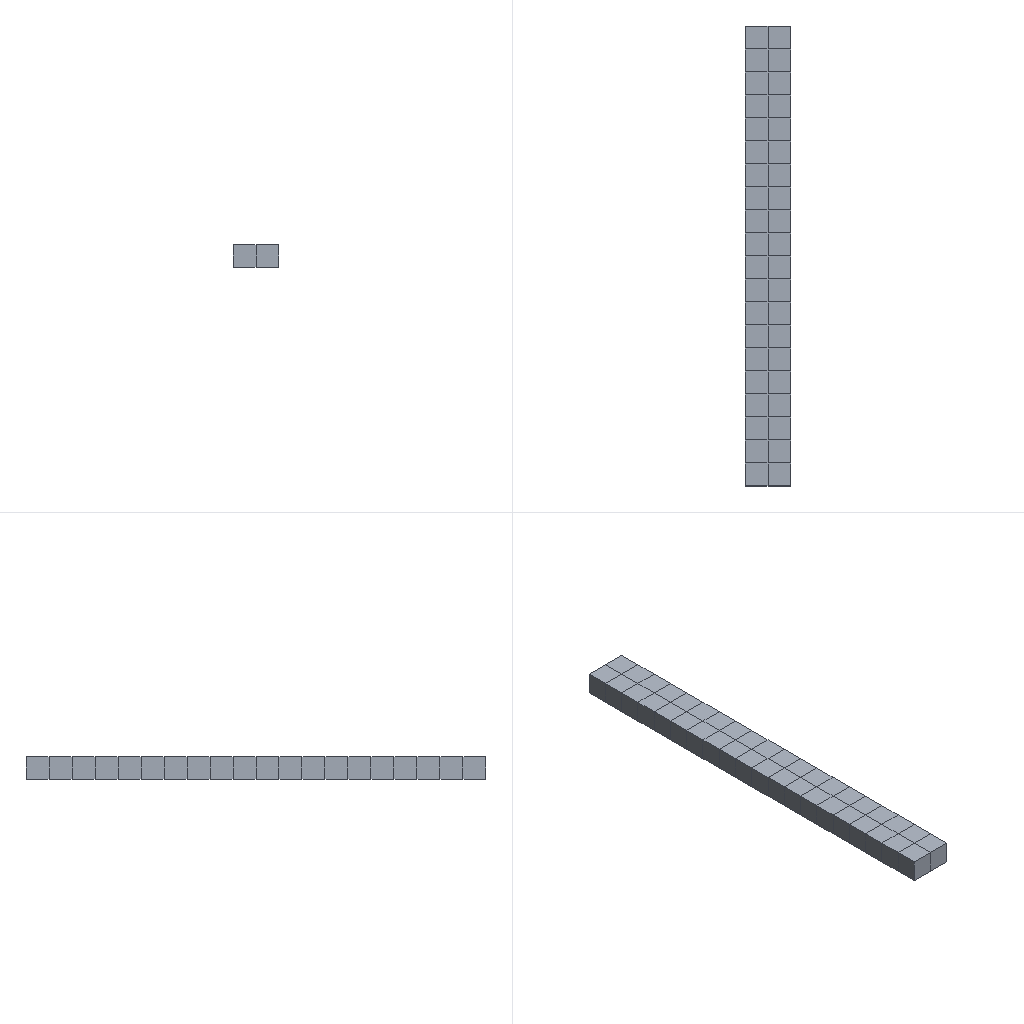Simulation study | ansys workbench
Ansys APDL input file, long lists of numbers shortened:
/batch
/config,noeldb,1     ! force off writing results to database
*get,_wallstrt,active,,time,wall
! ANSYS input file written by Workbench version 2022 R1
! File used for geometry attach: C:\Users\Administrator\AppData\Local\Temp\WB_Administrator_19516_2\wbnew_files\dp0\SYS\DM\SYS.scdoc
/title,wbnew--____ (A5)
! ****** Begin Custom Load Command Snippet ******
/COM, ACT Extensions:
/COM,     LSDYNA, 2021.1
/COM,
! ****** End   Custom Load Command Snippet ******
*DIM,_wb_ProjectScratch_dir,string,248
_wb_ProjectScratch_dir(1) = 'C:\Users\Administrator\AppData\Local\Temp\WB_Administrator_19516_2\_ProjectScratch\Scr58CE\'
*DIM,_wb_SolverFiles_dir,string,248
_wb_SolverFiles_dir(1) = 'C:\Users\Administrator\AppData\Local\Temp\WB_Administrator_19516_2\wbnew_files\dp0\SYS\MECH\'
*DIM,_wb_userfiles_dir,string,248
_wb_userfiles_dir(1) = 'C:\Users\Administrator\AppData\Local\Temp\WB_Administrator_19516_2\wbnew_files\user_files\'
/com,--- Data in consistent NMM units. See Solving Units in the help system for more information.
/units,MPA
/nopr
/wb,file,start              !  signify a WB generated input file
/prep7
! Turn off shape checking because checks already performed inside WB mesher.
! See help system for more information.
SHPP,OFF,,NOWARN
/nolist
etcon,set             ! allow ANSYS to choose best KEYOP's for 180x elements, resets any applicable keyopt to MAPDL defaults
/com,*********** Nodes for the whole assembly ***********
nblock,3,,1377
(1i9,3e20.9e3)
        1    -1.000000000E+01     6.000000000E+02    -3.572850612E-16
! (1251 more lines like these left out)
-1
/wb,elem,start            !  set before creation of elements
/com,*********** Elements for Body 1 "SYS\__" ***********
et,1,187
eblock,19,solid,,552
(19i9)
        1        1        1        1        0        0        0        0       10        0        1       86      230       90       95      641      658      637      638
! (1103 more lines like these left out)
-1
/wb,elem,end               !  done creating elements
/com,*********** Send User Defined Coordinate System(s) ***********
csys,0
toffst,273.15,  ! Temperature offset from absolute zero
/com,*********** Set Reference Temperature ***********
tref,22.
/wb,mat,start              !  starting to send materials
/com,*********** Send Materials ***********
Temperature = 'TEMP' ! Temperature
MP,DENS,1,7.85e-09,	! tonne mm^-3
MP,ALPX,1,1.2e-05,	! C^-1
MP,C,1,434000000,	! mm^2 s^-2 C^-1
MP,KXX,1,60.5,	! tonne mm s^-3 C^-1
MP,RSVX,1,0.00017,	! ohm mm
MP,EX,1,200000,	! tonne s^-2 mm^-1
MP,NUXY,1,0.3,
MP,MURX,1,10000,
/wb,mat,end                !  done sending materials
!************************* Model Summary ********************
!SYS\__,	结构钢,	matid,	1
!************************* End Model Summary ********************
! get the diagonal of the bounding box. Needed later for other things
*get,_xmin,node,,mnloc,x
*get,_ymin,node,,mnloc,y
*get,_zmin,node,,mnloc,z
*get,_xmax,node,,mxloc,x
*get,_ymax,node,,mxloc,y
*get,_zmax,node,,mxloc,z
_ASMDIAG=(_xmax-_xmin)*(_xmax-_xmin)+(_ymax-_ymin)*(_ymax-_ymin)+(_zmax-_zmin)*(_zmax-_zmin)
_ASMDIAG=SQRT(_ASMDIAG)
/wb,contact,start          !  starting to send contact
/wb,contact,end            !  done creating contacts
/golist
/wb,load,start             !  starting to send loads
/com,*********** Fixed Supports ***********
CMBLOCK,_FIXEDSU,NODE,       32
(8i10)
         1         2         3         4         5         6         7         8
        27        28        29        30        31        32        33        34
       239       240       243       244       250       251       256       257
       370       371       376       377       381       382       388       389
cmsel,s,_FIXEDSU
d,all,all
nsel,all
/com,******* Constant Zero Displacement X *******
CMBLOCK,_DISPZEROUX,NODE,       20
(8i10)
         9        10        11        12        13        14        15        16
        17        18       274       275       278       279       283       284
       290       291       297       298
cmsel,s,_DISPZEROUX
d,all,ux,0
nsel,all
/com,******* Constant Zero Displacement Z *******
CMBLOCK,_DISPZEROUZ,NODE,       20
(8i10)
         9        10        11        12        13        14        15        16
        17        18       274       275       278       279       283       284
       290       291       297       298
cmsel,s,_DISPZEROUZ
d,all,uz,0
nsel,all
/com,*********** Define Force Using Surface Effect Elements ***********
local,12,0,0.,0.,0.,0.,0.,0.
csys,0
et,2,154
eblock,10,,,6
(15i9)
     1003        2        2        2       12       31       34       28       28      392      378       28      376
     1004        2        2        2       12       27       34       31       31      371      392       31      370
     1005        2        2        2       12       29       32       33       33      381      397       33      382
     1006        2        2        2       12       34       30       32       32      389      387       32      398
     1007        2        2        2       12       32       30       33       33      387      388       33      397
     1008        2        2        2       12       28       34       32       32      378      398       32      377
-1
esel,s,type,,2
keyop,2,2,1                ! Apply load in local coordinate system
keyop,2,7,1                ! Use original area so load is constant in large deformation
esel,all
/com,*********** Define Force Using Surface Effect Elements ***********
local,13,0,0.,0.,0.,0.,0.,0.
csys,0
et,3,154
eblock,10,,,6
(15i9)
     1009        3        3        3       13        6        2        7        7      244      245        7      264
     1010        3        3        3       13        7        2        5        5      245      243        5      259
     1011        3        3        3       13        7        5        4        4      259      255        4      256
     1012        3        3        3       13        3        6        7        7      250      264        7      251
     1013        3        3        3       13        1        8        5        5      240      260        5      239
     1014        3        3        3       13        4        5        8        8      255      260        8      257
-1
esel,s,type,,3
keyop,3,2,1                ! Apply load in local coordinate system
keyop,3,7,1                ! Use original area so load is constant in large deformation
esel,all
/com,*********** Define Force Using Surface Effect Elements ***********
local,14,0,0.,0.,0.,0.,0.,0.
csys,0
et,4,154
eblock,10,,,18
(15i9)
     1015        4        4        4       14       11       15       25       25      283      307       25      286
! (17 more lines like these left out)
-1
esel,s,type,,4
keyop,4,2,1                ! Apply load in local coordinate system
keyop,4,7,1                ! Use original area so load is constant in large deformation
esel,all
/gst,on,on
fini
*get,_numnode,node,0,count
*get,_numelem,elem,0,count
*get, _MAXELEMNUM, elem, 0, NUM, MAX
*get, _MAXNODENUM, node, 0, NUM, MAX
*get, _MAXELEMTYPE, etyp, 0, NUM, MAX
*get, _MAXREALCONST, real, 0, NUM, MAX
/go
/wb,load,end               !  done creating loads
/com,--- Number of total nodes = %_numnode%
/com,--- Number of contact elements = 30
/com,--- Number of spring elements = 0
/com,--- Number of bearing elements = 0
/com,--- Number of solid elements = 552
/com,--- Number of condensed parts = 0
/com,--- Number of total elements = %_numelem%
*get,_wallbsol,active,,time,wall
/com,****************************************************************************
/com,*************************    SOLUTION       ********************************
/com,****************************************************************************
/solu
antype,0                   ! static analysis
_thickRatio=  0     ! Ratio of thick parts in the model
eqsl,sparse,,,,,1
cntr,print,1               ! print out contact info and also make no initial contact an error
dmpoption,emat,no             ! Don't combine emat file for DANSYS
dmpoption,esav,no             ! Don't combine esav file for DANSYS
nldiag,cont,iter           ! print out contact info each equilibrium iteration
rescontrol,,none                 ! Do not keep any restart files
/com,****************************************************
/com,******************* SOLVE FOR LS 1 OF 1 ****************
esel,s,type,,2
nsle
sfe,all,1,pres,1,0.
sfe,all,2,pres,1,-513.134
sfe,all,3,pres,1,0.
esel,s,type,,3
nsle
sfe,all,1,pres,1,0.
sfe,all,2,pres,1,-192.437
sfe,all,3,pres,1,0.
esel,s,type,,4
nsle
sfe,all,1,pres,1,0.
sfe,all,2,pres,1,4244.847
sfe,all,3,pres,1,0.
nsel,all
esel,all
/nopr
/gopr
nsub,1,1,1
time,1.
outres,erase
outres,all,none
outres,nsol,all,
outres,rsol,all
outres,eangl,all
outres,etmp,all
outres,veng,all
outres,strs,all,
outres,epel,all,
outres,eppl,all,
outres,cont,all,
! *********** WB SOLVE COMMAND ***********
! check interactive state
*get,ANSINTER_,active,,int
*if,ANSINTER_,ne,0,then
/eof
*endif
solve
/com *************** Write FE CONNECTORS *********
CEWRITE,file,ce,,INTE
/com,****************************************************
/com,*************** FINISHED SOLVE FOR LS 1 *************
*get,_wallasol,active,,time,wall
/nopr
*get,_numnode,node,0,count
*get,_numelem,elem,0,count
*get, _MAXELEMNUM, elem, 0, NUM, MAX
*get, _MAXNODENUM, node, 0, NUM, MAX,,,INTERNAL
*get, _MAXELEMTYPE, etyp, 0, NUM, MAX
*get, _MAXREALCONST, real, 0, NUM, MAX
/gopr
/post1
xmlo,ENCODING,ISO-8859-1
xmlo,parm
/xml,parm,xml
fini
/gopr
*get,_walldone,active,,time,wall
_preptime=(_wallbsol-_wallstrt)*3600
_solvtime=(_wallasol-_wallbsol)*3600
_posttime=(_walldone-_wallasol)*3600
_totaltim=(_walldone-_wallstrt)*3600
*get,_dlbratio,active,0,solu,dlbr
*get,_combtime,active,0,solu,comb
*get,_ssmode,active,0,solu,ssmm
*get,_ndofs,active,0,solu,ndof
*get,_sol_end_time,active,0,set,time
*if,_sol_end_time,eq,1.,then
/fclean				!clean distributed files
*endif
/com,--- Total number of nodes = %_numnode%
/com,--- Total number of elements = %_numelem%
/com,--- Element load balance ratio = %_dlbratio%
/com,--- Time to combine distributed files = %_combtime%
/com,--- Sparse memory mode = %_ssmode%
/com,--- Number of DOF = %_ndofs%
/wb,file,end               ! done with WB generated input